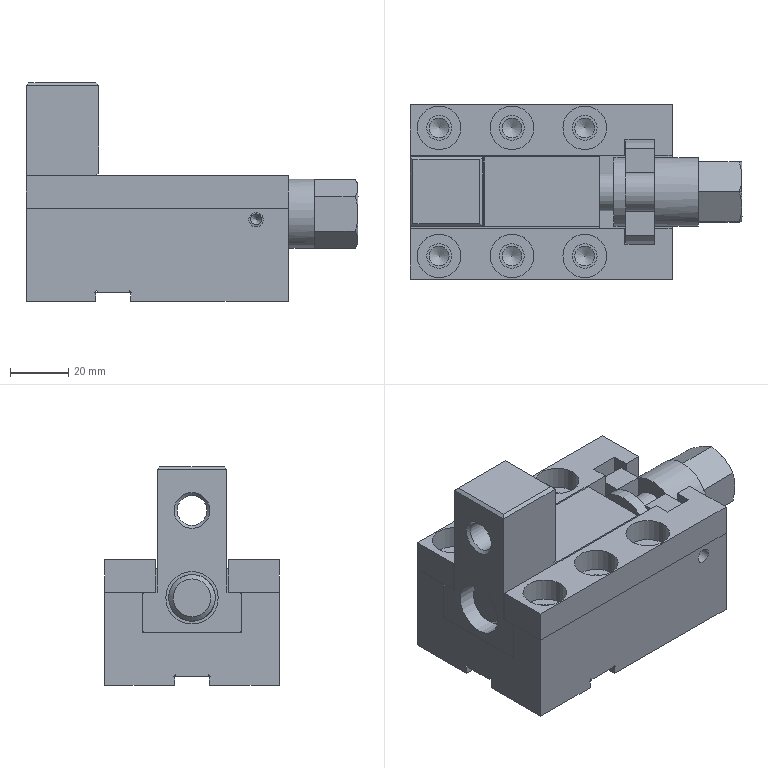Part | NX | features DATUM_CSYS 37, SKETCH 30, EXTRUDE 22, EXTRACT_FACE 14, EXTRACT_STRING 12, HOLE PACKAGE 12, SIMPLE HOLE 12, SYMBOLIC_THREAD 12, Instance Feature 10, CYLINDER 9, BLOCK 7, CHAMFER 5, Pattern Feature 4, CONE 2, RECT_SLOT 2, SKIN 2, BLEND 1, CPROJ 1, DATUM_ON_PATH 1, DATUM_PLANE 1, MIRROR_SET 1, THREADS 1, TRIM BODY 1 | 8 solids | 217 faces | box 114 x 60 x 75 mm | volume 223844 mm3 | plane 143 | cylinder 52 | cone 12 | spline 10 | commonest cylinder face diameters 1 x8 6.8 x6 8.5 x6 15 x6 36 x4 11 x3